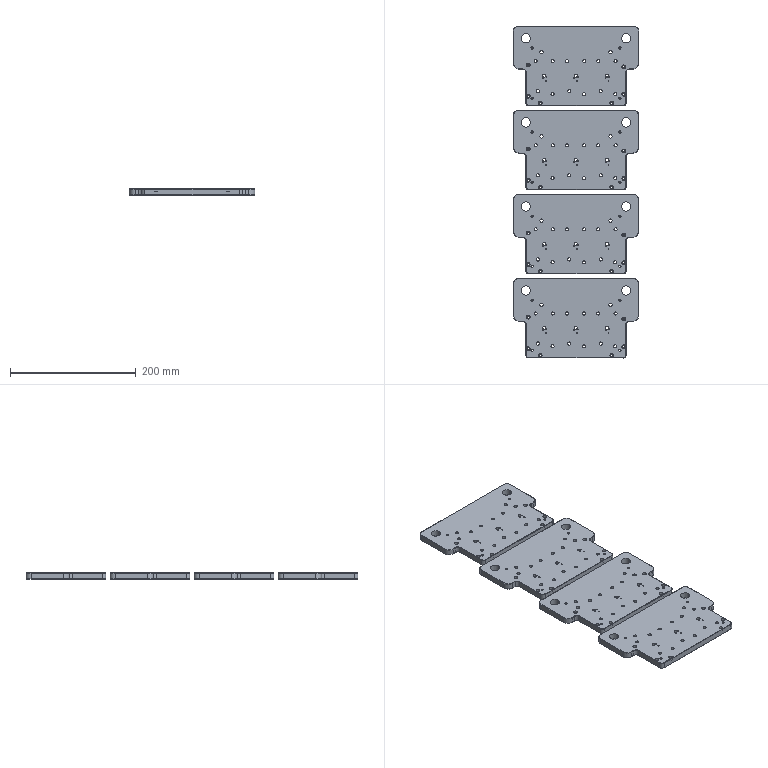Part | 4 solids | 672 faces | box 200 x 529 x 10 mm | volume 884426 mm3 | cylinder 456 | plane 152 | cone 64 | commonest cylinder face diameters 5 x136 3.5 x80 1 x72 6 x64 6.5 x32 1.7 x24